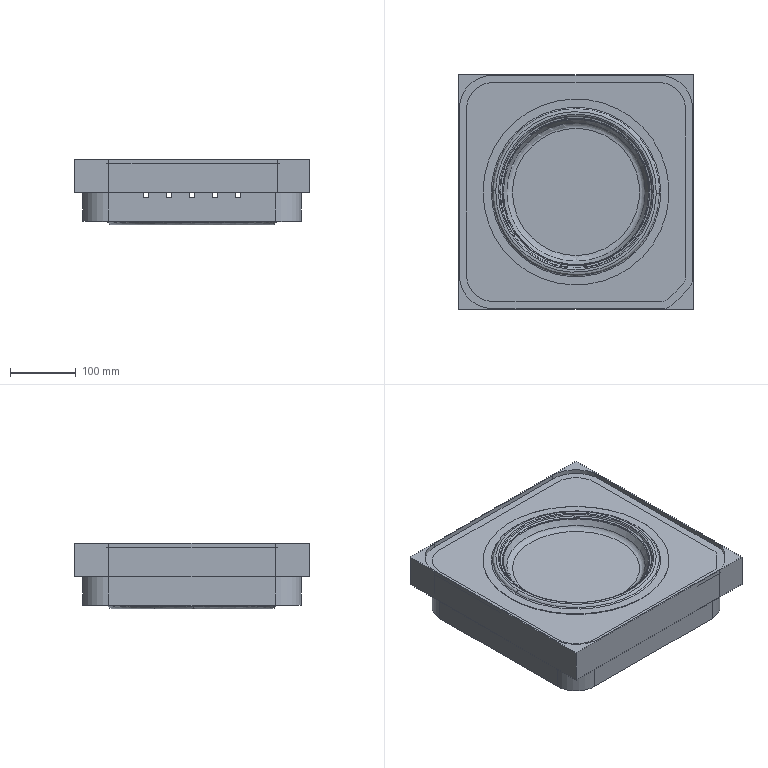NC program | NX | posted with a generic post | part box 356 x 356 x 99.5 mm
Lines 5552 to 6475 of 165566:
(06 , TOOL : R2)
N11090 M6
N11092 G53
N11094 G17 G0 G90 X-7.96 Y-140.743 S8000 M3 M8
N11096 G43 Z200.5 H0
N11098 Z47.725
N11100 G94 G1 Z44.725 F4500.
N11102 X-8.307 Y-140.727
N11104 X-8.475 Y-140.721
N11106 X-10.032 Y-140.636
N11108 G2 X-20.418 Y-139.492 R132.954
N11110 G1 X-21.112 Y-139.397
N11112 X-21.594 Y-139.336
N11114 X-26.993 Y-138.383
N11116 X-27.456 Y-138.297
N11118 X-32.877 Y-137.105
N11120 X-33.572 Y-136.93
N11122 X-33.644 Y-136.913
N11124 X-37.606 Y-135.874
N11126 X-38.416 Y-135.657
N11128 X-38.877 Y-135.528
N11130 X-42.571 Y-134.392
N11132 X-43.388 Y-134.143
N11134 X-43.954 Y-133.964
N11136 X-44.464 Y-133.797
N11138 X-49.379 Y-132.066
N11140 X-50.266 Y-131.72
N11142 X-50.877 Y-131.476
N11144 X-53.992 Y-130.232
N11146 G2 X-57.735 Y-128.604 R67.091
N11148 G1 X-60.048 Y-127.566
N11150 X-60.222 Y-127.485
N11152 X-60.567 Y-127.317
N11154 X-65.412 Y-124.904
N11156 X-65.76 Y-124.713
N11158 X-68.399 Y-123.263
N11160 X-69.566 Y-122.621
N11162 X-70.632 Y-122.027
N11164 X-71.206 Y-121.68
N11166 X-75.449 Y-119.111
N11168 X-76.798 Y-118.218
N11170 X-77.32 Y-117.873
N11172 X-77.841 Y-117.527
N11174 X-78.22 Y-117.277
N11176 X-78.889 Y-116.834
N11178 X-78.913 Y-116.818
N11180 X-79.93 Y-116.145
N11182 X-80.442 Y-115.796
N11184 X-82.356 Y-114.411
N11186 X-84.747 Y-112.68
N11188 X-85.207 Y-112.334
N11190 X-86.523 Y-111.293
N11192 X-87.216 Y-110.748
N11194 X-88.28 Y-109.911
N11196 X-89.16 Y-109.218
N11198 X-89.592 Y-108.872
N11200 X-90.603 Y-108.006
N11202 X-93.632 Y-105.41
N11204 X-94.026 Y-105.064
N11206 X-94.142 Y-104.957
N11208 X-94.772 Y-104.37
N11210 X-95.492 Y-103.701
N11212 X-95.869 Y-103.35
N11214 X-96.217 Y-103.026
N11216 X-96.259 Y-102.987
N11218 X-98.119 Y-101.256
N11220 X-102.231 Y-97.102
N11222 X-102.746 Y-96.538
N11224 X-105.074 Y-93.985
N11226 X-106.021 Y-92.948
N11228 X-106.601 Y-92.267
N11230 X-107.77 Y-90.874
N11232 X-109.802 Y-88.448
N11234 X-111.945 Y-85.679
N11236 X-113.279 Y-83.947
N11238 X-113.529 Y-83.608
N11240 X-113.778 Y-83.255
N11242 X-114.519 Y-82.209
N11244 X-115.248 Y-81.179
N11246 X-115.253 Y-81.172
N11248 X-116.227 Y-79.794
N11250 X-116.717 Y-79.101
N11252 X-119.859 Y-74.255
N11254 X-120.476 Y-73.216
N11256 X-121.829 Y-70.929
N11258 X-121.909 Y-70.793
N11260 X-121.959 Y-70.708 Z44.724
N11262 X-122.108 Y-70.453 Z44.725
N11264 X-122.174 Y-70.344
N11266 X-122.518 Y-69.76
N11268 X-122.867 Y-69.164
N11270 X-122.921 Y-69.062
N11272 X-123.906 Y-67.231
N11274 X-124.965 Y-65.254
N11276 X-125.522 Y-64.216
N11278 X-125.691 Y-63.878
N11280 X-128.048 Y-59.023
N11282 X-128.654 Y-57.639
N11284 X-130.312 Y-53.83
N11286 X-130.478 Y-53.432
N11288 X-131.665 Y-50.369
N11290 X-132.466 Y-48.291
N11292 X-132.591 Y-47.945
N11294 X-134.357 Y-42.753
N11296 X-135.18 Y-39.983
N11298 X-135.877 Y-37.62
N11300 X-135.996 Y-37.214
N11302 X-136.016 Y-37.139
N11304 X-137.392 Y-31.675
N11306 X-137.402 Y-31.632
N11308 X-138.548 Y-26.136
N11310 X-138.673 Y-25.444
N11312 X-139.133 Y-22.68
N11314 X-139.475 Y-20.597
N11316 X-139.495 Y-20.562
N11318 X-140.18 Y-15.059
N11320 X-140.26 Y-14.366
N11322 X-140.717 Y-8.827
N11324 X-140.738 Y-8.481
N11326 X-140.794 Y-7.097
N11328 X-140.865 Y-5.468
N11330 Y-5.366
N11332 X-140.88 Y-5.02
N11334 X-140.881 Y-5.012
N11336 X-140.896 Y-4.673
N11338 X-140.965 Y-2.942
N11340 X-140.982 Y-1.558
N11342 X-140.989 Y-0.865
N11344 X-140.994 Y-0.173
N11346 X-140.993 Y0.516
N11348 X-140.985 Y1.212
N11350 X-140.978 Y1.904
N11352 X-140.965 Y2.934
N11354 X-140.951 Y3.289
N11356 G3 X-140.738 Y8.477 R4785.324
N11358 G1 X-140.691 Y9.172
N11360 X-140.261 Y14.355
N11362 G2 X-139.475 Y20.597 R236.107
N11364 G1 X-138.731 Y25.098
N11366 X-138.614 Y25.788
N11368 X-138.549 Y26.131
N11370 X-137.404 Y31.632
N11372 X-137.219 Y32.366
N11374 X-136.017 Y37.136
N11376 X-135.996 Y37.214
N11378 X-135.895 Y37.56
N11380 X-135.086 Y40.303
N11382 X-134.358 Y42.748
N11384 X-132.558 Y48.043
N11386 X-132.336 Y48.637
N11388 X-130.481 Y53.425
N11390 X-130.313 Y53.828
N11392 X-128.204 Y58.675
N11394 X-128.052 Y59.014
N11396 X-127.209 Y60.753
N11398 X-125.982 Y63.28
N11400 X-125.636 Y63.994
N11402 X-125.521 Y64.213
N11404 X-124.966 Y65.254
N11406 X-122.867 Y69.165
N11408 X-122.726 Y69.407
N11410 X-120.45 Y73.261
N11412 X-119.86 Y74.253
N11414 X-116.718 Y79.1
N11416 X-116.29 Y79.706
N11418 X-115.599 Y80.686
N11420 X-115.491 Y80.833
N11422 X-114.56 Y82.152
N11424 X-113.867 Y83.13
N11426 X-113.525 Y83.613
N11428 X-113.176 Y84.083
N11430 X-112.484 Y84.981
N11432 X-112.479 Y84.986
N11434 X-110.072 Y88.1
N11436 X-109.971 Y88.23 Z44.723
N11438 X-109.801 Y88.448 Z44.725
N11440 X-107.293 Y91.443
N11442 X-107.19 Y91.564
N11444 X-106.946 Y91.855
N11446 X-106.611 Y92.253
N11448 X-106.254 Y92.678
N11450 X-106.021 Y92.947
N11452 X-105.907 Y93.072
N11454 X-105.074 Y93.987
N11456 X-104.178 Y94.97
N11458 X-102.867 Y96.408
N11460 X-102.447 Y96.87
N11462 X-102.101 Y97.237
N11464 X-98.12 Y101.255
N11466 X-94.487 Y104.637
N11468 X-94.027 Y105.064
N11470 X-93.449 Y105.566
N11472 X-92.756 Y106.162
N11474 X-89.592 Y108.872
N11476 X-88.722 Y109.565
N11478 X-86.964 Y110.948
N11480 X-86.872 Y111.02
N11482 X-85.042 Y112.458 Z44.723
N11484 X-84.796 Y112.642 Z44.725
N11486 X-84.795 Y112.643
N11488 X-82.356 Y114.411
N11490 X-81.357 Y115.132
N11492 X-80.296 Y115.898
N11494 X-75.451 Y119.11
N11496 X-75.105 Y119.319
N11498 X-72.976 Y120.609
N11500 X-72.352 Y120.988
N11502 X-70.605 Y122.043
N11504 X-66.874 Y124.104
N11506 X-66.287 Y124.425
N11508 X-66.106 Y124.526
N11510 X-66.012 Y124.577 Z44.724
N11512 X-65.76 Y124.714 Z44.725
N11514 X-65.414 Y124.903
N11516 X-60.915 Y127.144
N11518 X-60.568 Y127.316
N11520 X-60.056 Y127.562
N11522 X-56.961 Y128.951
N11524 X-56.416 Y129.194
N11526 X-55.39 Y129.653
N11528 X-54.603 Y129.989
N11530 X-50.877 Y131.476
N11532 X-49.38 Y132.063
N11534 X-49.146 Y132.147
N11536 X-46.432 Y133.105
N11538 X-44.301 Y133.851
N11540 X-43.387 Y134.143
N11542 X-39.456 Y135.348
N11544 X-38.763 Y135.56
N11546 X-38.072 Y135.75
N11548 X-37.379 Y135.933
N11550 X-35.306 Y136.475
N11552 X-33.918 Y136.842
N11554 X-32.88 Y137.105
N11556 X-27.456 Y138.297
N11558 X-26.996 Y138.383
N11560 X-24.227 Y138.871
N11562 X-22.843 Y139.114
N11564 X-21.593 Y139.336
N11566 X-21.115 Y139.396
N11568 X-16.267 Y140.05
N11570 X-15.575 Y140.128
N11572 X-10.729 Y140.579
N11574 X-10.037 Y140.635
N11576 X-8.474 Y140.721
N11578 X-7.963 Y140.743
N11580 X-7.268 Y140.78
N11582 X-6.23 Y140.833
N11584 X-4.499 Y140.919
N11586 X-3.807 Y140.936
N11588 X-2.769 Y140.946
N11590 X1.038 Y140.986
N11592 X1.384 Y140.983
N11594 X1.726 Y140.977
N11596 X6.23 Y140.845
N11598 X6.918 Y140.822
N11600 X7.609 Y140.784
N11602 X8.534 Y140.721
N11604 X8.999 Y140.684
N11606 X9.345 Y140.659
N11608 X10.383 Y140.585
N11610 X11.768 Y140.484
N11612 X12.791 Y140.411
N11614 X13.221 Y140.374
N11616 X18.681 Y139.751
N11618 X19.171 Y139.682
N11620 X24.224 Y138.896
N11622 X24.57 Y138.836
N11624 X26.302 Y138.496
N11626 X30.105 Y137.743
N11628 X30.706 Y137.605
N11630 X35.646 Y136.413
N11632 X35.99 Y136.322
N11634 X36.341 Y136.22
N11636 X36.357 Y136.219
N11638 X36.375 Y136.215
N11640 X41.224 Y134.836
N11642 X42.291 Y134.491
N11644 X46.489 Y133.105
N11646 X47.46 Y132.759
N11648 X50.185 Y131.736
N11650 X52.057 Y131.028
N11652 X52.91 Y130.681
N11654 X53.727 Y130.334
N11656 X56.152 Y129.31
N11658 X57.778 Y128.614
N11660 X57.794 Y128.604
N11662 X58.149 Y128.437
N11664 X59.532 Y127.783
N11666 X62.191 Y126.526
N11668 X62.915 Y126.181
N11670 X64.24 Y125.489
N11672 X67.536 Y123.762
N11674 X68.183 Y123.412
N11676 X72.979 Y120.642
N11678 X73.72 Y120.172
N11680 X77.893 Y117.528
N11682 X78.398 Y117.18
N11684 X79.398 Y116.487
N11686 X79.896 Y116.141
N11688 X82.717 Y114.183
N11690 X82.875 Y114.064
N11692 X83.397 Y113.67
N11694 X87.002 Y110.949
N11696 X87.44 Y110.603
N11698 X87.911 Y110.216
N11700 X89.127 Y109.217
N11702 X89.968 Y108.526
N11704 X91.653 Y107.141
N11706 X92.047 Y106.795
N11708 X94.833 Y104.308
N11710 X95.149 Y104.026
N11712 X95.175 Y104.002
N11714 X95.925 Y103.333
N11716 X96.216 Y103.063
N11718 X100.218 Y99.179
N11720 X102.847 Y96.41
N11722 X104.167 Y95.025
N11724 X107.492 Y91.225
N11726 X108.097 Y90.525
N11728 X111.44 Y86.372
N11730 X111.71 Y86.024
N11732 X113.247 Y83.948
N11734 X115.036 Y81.524
N11736 X115.252 Y81.216
N11738 X115.512 Y80.831
N11740 X115.945 Y80.194
N11742 X118.365 Y76.614
N11744 X119.406 Y74.936
N11746 X119.54 Y74.718
N11748 X121.324 Y71.832
N11750 X121.526 Y71.485
N11752 X124.256 Y66.639
N11754 X124.341 Y66.471 Z44.722
N11756 X124.43 Y66.294 Z44.725
N11758 X124.608 Y65.947
N11760 X125.49 Y64.22
N11762 X126.728 Y61.792
N11764 X127.02 Y61.192
N11766 X128.55 Y57.865
N11768 X128.972 Y56.945
N11770 X129.284 Y56.254
N11772 X130.135 Y54.198
N11774 X130.142 Y54.177
N11776 X130.286 Y53.83
N11778 X131.282 Y51.407
N11780 X131.558 Y50.715
N11782 X132.061 Y49.33
N11784 X132.439 Y48.292
N11786 X132.903 Y47.015
N11788 X133.164 Y46.302
N11790 X133.25 Y46.063
N11792 X133.443 Y45.522
N11794 X133.779 Y44.484
N11796 X134.992 Y40.675
N11798 X135.206 Y39.983
N11800 X135.672 Y38.296
N11802 X136.712 Y34.498
N11804 X136.806 Y34.098
N11806 X137.996 Y28.906
N11808 X138.096 Y28.435
N11810 X139.04 Y23.367
N11812 X139.101 Y23.021
N11814 X139.132 Y22.833
N11816 X139.605 Y19.559
N11818 X139.905 Y17.482
N11820 X139.948 Y17.136
N11822 X140.519 Y11.597
N11824 X140.821 Y6.75
N11826 X140.859 Y6.058
N11828 X140.876 Y6.031
N11830 X140.988 Y0.519
N11832 X140.987 Y-0.512
N11834 X140.918 Y-3.824
N11836 X140.873 Y-6.04
N11838 X140.865 Y-6.053
N11840 X140.859 Y-6.058
N11842 X140.68 Y-9.
N11844 X140.519 Y-11.597
N11846 X140.34 Y-13.328
N11848 X139.949 Y-17.13
N11850 X139.906 Y-17.475
N11852 X139.274 Y-21.846
N11854 X139.132 Y-22.83
N11856 X139.101 Y-23.021
N11858 X138.264 Y-27.521
N11860 X138.097 Y-28.43
N11862 X137.997 Y-28.903
N11864 X137.841 Y-29.596
N11866 X137.523 Y-30.983
N11868 X136.712 Y-34.496
N11870 X135.329 Y-39.553
N11872 X135.206 Y-39.981
N11874 X135.1 Y-40.33
N11876 X133.944 Y-43.964
N11878 X133.444 Y-45.52
N11880 X133.321 Y-45.868
N11882 X133.113 Y-46.437
N11884 X131.935 Y-49.676
N11886 X131.558 Y-50.714
N11888 X131.282 Y-51.407
N11890 X129.576 Y-55.553
N11892 X129.285 Y-56.251
N11894 X128.972 Y-56.946
N11896 X128.653 Y-57.641
N11898 X128.201 Y-58.625
N11900 X127.021 Y-61.191
N11902 X126.901 Y-61.445
N11904 X126.674 Y-61.906
N11906 X126.555 Y-62.139
N11908 X124.255 Y-66.641
N11910 X124.062 Y-66.985
N11912 X123.477 Y-68.024
N11914 X121.525 Y-71.48
N11916 X121.325 Y-71.83
N11918 X121.134 Y-72.14
N11920 X120.899 Y-72.523
N11922 X120.445 Y-73.259
N11924 X120.327 Y-73.448
N11926 X119.827 Y-74.255
N11928 X119.406 Y-74.935
N11930 X118.368 Y-76.612
N11932 X116.637 Y-79.171
N11934 X116.214 Y-79.794
N11936 X115.945 Y-80.193
N11938 X115.512 Y-80.831
N11940 X115.253 Y-81.215
N11942 X115.036 Y-81.524
N11944 X114.561 Y-82.173
N11946 X112.483 Y-84.982
N11948 X111.792 Y-85.916
N11950 X111.445 Y-86.367
N11952 X108.098 Y-90.524
N11954 X107.985 Y-90.66
N11956 X106.6 Y-92.243
N11958 X104.524 Y-94.619
N11960 X104.47 Y-94.679
N11962 X104.177 Y-95.014
N11964 X100.219 Y-99.179
N11966 X96.217 Y-103.062
N11968 X95.925 Y-103.334
N11970 X95.871 Y-103.382
N11972 X91.718 Y-107.087
N11974 X91.074 Y-107.62
N11976 X89.711 Y-108.739
N11978 X88.603 Y-109.651
N11980 X87.218 Y-110.781
N11982 X86.542 Y-111.296
N11984 X85.169 Y-112.334
N11986 X82.719 Y-114.182
N11988 X81.743 Y-114.861
N11990 X81.335 Y-115.144
N11992 X79.894 Y-116.142
N11994 X78.912 Y-116.823
N11996 X78.566 Y-117.062
N11998 X78.55 Y-117.073
N12000 X77.895 Y-117.527
N12002 X77.874 Y-117.541
N12004 X77.734 Y-117.63 Z44.722
N12006 X77.531 Y-117.759 Z44.725
N12008 X72.98 Y-120.642
N12010 X69.57 Y-122.611
N12012 X68.848 Y-123.027
N12014 X68.183 Y-123.412
N12016 X67.151 Y-123.963
N12018 X62.991 Y-126.142
N12020 X62.916 Y-126.179
N12022 G2 X57.454 Y-128.756 R593.172
N12024 G1 X56.415 Y-129.198
N12026 X53.646 Y-130.368
N12028 X52.914 Y-130.68
N12030 X52.495 Y-130.853
N12032 X52.262 Y-130.948
N12034 X52.07 Y-131.023
N12036 X50.531 Y-131.605
N12038 X47.07 Y-132.901
N12040 X46.724 Y-133.024
N12042 X46.499 Y-133.101
N12044 X44.393 Y-133.795
N12046 X42.917 Y-134.284
N12048 X41.224 Y-134.836
N12050 X36.357 Y-136.219
N12052 X36.341 Y-136.22
N12054 X35.995 Y-136.321
N12056 X35.649 Y-136.412
N12058 X35.021 Y-136.566
N12060 X30.711 Y-137.604
N12062 X30.111 Y-137.742
N12064 X24.573 Y-138.836
N12066 X23.638 Y-138.989
N12068 X19.382 Y-139.649
N12070 X19.172 Y-139.68
N12072 X18.69 Y-139.75
N12074 X14.883 Y-140.184
N12076 X14.19 Y-140.261
N12078 X13.222 Y-140.374
N12080 X12.806 Y-140.41
N12082 X7.614 Y-140.784
N12084 X6.922 Y-140.822
N12086 X6.23 Y-140.845
N12088 X1.731 Y-140.977
N12090 X1.384 Y-140.983
N12092 X1.038 Y-140.986
N12094 X-3.805 Y-140.936
N12096 X-4.497 Y-140.92
N12098 X-7.96 Y-140.743
N12100 Y-140.458
N12102 X-8.626 Y-140.427
N12104 G2 X-16.594 Y-139.719 R116.439
N12106 G1 X-21.487 Y-139.061
N12108 X-26.996 Y-138.092
N12110 X-27.342 Y-138.028
N12112 G2 X-49.482 Y-131.72 R141.758
N12114 G1 X-50.185 Y-131.445
N12116 G2 X-70.605 Y-121.71 R138.589
N12118 G1 X-71.797 Y-120.989
N12120 X-72.133 Y-120.786
N12122 X-75.227 Y-118.911
N12124 G2 X-102.101 Y-96.821 R141.205
N12126 G1 X-102.628 Y-96.245
N12128 X-105.764 Y-92.804
N12130 X-106.529 Y-91.91
N12132 X-109.419 Y-88.463
N12134 X-109.559 Y-88.291
N12136 X-109.709 Y-88.102
N12138 X-112.064 Y-85.057
N12140 X-113.176 Y-83.606
N12142 X-114.899 Y-81.178
N12144 X-115.045 Y-80.973
N12146 X-116.353 Y-79.122
N12148 X-116.478 Y-78.941
N12150 X-116.602 Y-78.755
N12152 X-119.609 Y-74.112
N12154 X-120.91 Y-71.925
N12156 X-121.578 Y-70.793
N12158 X-121.829 Y-70.366
N12160 X-122.596 Y-69.062
N12162 X-125.29 Y-64.042
N12164 X-126.701 Y-61.147
N12166 X-127.053 Y-60.423
N12168 X-127.722 Y-59.042
N12170 X-127.838 Y-58.795
N12172 G2 X-134.056 Y-42.753 R142.682
N12174 G1 X-135.29 Y-38.599
N12176 X-135.7 Y-37.214
N12178 X-136.187 Y-35.304
N12180 X-137.099 Y-31.675
N12182 G2 X-140.452 Y-8.481 R142.554
N12184 G1 X-140.455 Y-8.418
N12186 X-140.538 Y-6.427
N12188 X-140.592 Y-5.093
N12190 G2 X-140.583 Y5.302 R110.795
N12192 G1 X-140.58 Y5.366
N12194 X-140.57 Y5.675
N12196 X-140.447 Y8.553
N12198 X-140.394 Y9.298
N12200 X-139.989 Y14.204
N12202 X-139.853 Y15.384
N12204 X-139.235 Y20.35
N12206 X-139.187 Y20.597
N12208 X-139.178 Y20.65
N12210 X-138.442 Y25.095
N12212 X-138.295 Y25.937
N12214 X-137.827 Y28.213
N12216 X-137.1 Y31.67
N12218 X-135.771 Y36.944
N12220 X-135.702 Y37.207
N12222 X-134.109 Y42.587
N12224 X-133.25 Y45.124
N12226 G2 X-130. Y53.83 R125.039
N12228 G1 X-127.838 Y58.794
N12230 X-126.388 Y61.792
N12232 X-125.982 Y62.625
N12234 X-125.547 Y63.523
N12236 X-125.379 Y63.869
N12238 X-125.365 Y63.896
N12240 X-125.096 Y64.409
N12242 X-125.016 Y64.562
N12244 X-122.586 Y69.081
N12246 X-120.213 Y73.101
N12248 X-119.704 Y73.957
N12250 X-119.518 Y74.255
N12252 X-119.492 Y74.296
N12254 X-116.535 Y78.857
N12256 X-116.354 Y79.122
N12258 X-115.351 Y80.542
N12260 X-113.179 Y83.602
N12262 X-112.9 Y83.975
N12264 X-109.689 Y88.128
N12266 X-109.43 Y88.448
N12268 X-109.073 Y88.875
N12270 X-105.918 Y92.631
N12272 X-103.95 Y94.796
N12274 X-102.118 Y96.803
N12276 G2 X-91.577 Y106.795 R131.576
N12278 G1 X-90.132 Y108.035
N12280 X-89.415 Y108.649
N12282 X-88.663 Y109.247
N12284 G2 X-74.087 Y119.604 R134.667
N12286 G1 X-73.438 Y119.998
N12288 X-72.759 Y120.408
N12290 X-72.28 Y120.699
N12292 X-70.532 Y121.755
N12294 X-68.529 Y122.866
N12296 X-65.414 Y124.578
N12298 G2 X-10.441 Y140.316 R141.001
N12300 G1 X-10.064 Y140.347
N12302 X-8.339 Y140.441
N12304 G2 X7.73 Y140.49 R137.262
N12306 X19.036 Y139.413 R134.033
N12308 G1 X23.189 Y138.768
N12310 X23.535 Y138.715
N12312 X24.195 Y138.611
N12314 G2 X47.416 Y132.47 R139.657
N12316 G1 X49.186 Y131.807
N12318 X50.185 Y131.431
N12320 X52.165 Y130.681
N12322 X54.761 Y129.588
N12324 X57.584 Y128.391
N12326 G2 X77.874 Y117.196 R142.328
N12328 G1 X82.581 Y113.927
N12330 G2 X95.871 Y102.995 R142.11
N12332 G1 X100.072 Y98.919
N12334 X103.968 Y94.82
N12336 G2 X114.929 Y81.181 R142.124
N12338 G1 X115.061 Y80.987
N12340 X116.459 Y78.923
N12342 X116.752 Y78.491
N12344 X118.022 Y76.616
N12346 X118.142 Y76.431
N12348 X118.368 Y76.067
N12350 X119.326 Y74.521
N12352 X120.114 Y73.251
N12354 X120.252 Y73.024
N12356 X121.165 Y71.538
N12358 X123.298 Y67.761
N12360 X123.921 Y66.652
N12362 G2 X126.907 Y60.754 R133.035
N12364 G1 X127.051 Y60.443
N12366 X127.161 Y60.202
N12368 G2 X134.47 Y41.368 R134.33
N12370 G1 X134.691 Y40.681
N12372 X134.761 Y40.456
N12374 X134.981 Y39.727
N12376 X136.428 Y34.454
N12378 X137.389 Y30.29
N12380 X137.712 Y28.868
N12382 X137.777 Y28.565
N12384 X138.817 Y23.005
N12386 X139.616 Y17.482
N12388 X139.697 Y16.79
N12390 X140.232 Y11.602
N12392 X140.535 Y6.77
N12394 X140.571 Y6.114
N12396 X140.575 Y6.058
N12398 X140.595 Y5.789
N12400 G2 X140.571 Y-6.114 R144.764
N12402 G1 X140.317 Y-10.25
N12404 X140.237 Y-11.533
N12406 X140.232 Y-11.597
N12408 X139.66 Y-17.136
N12410 X139.561 Y-17.879
N12412 X138.818 Y-23.004
N12414 X137.78 Y-28.549
N12416 X137.548 Y-29.598
N12418 G2 X123.96 Y-66.585 R140.355
N12420 G1 X121.59 Y-70.793
N12422 X121.137 Y-71.585
N12424 X120.121 Y-73.239
N12426 X118.145 Y-76.431
N12428 X116.34 Y-79.101
N12430 X115.945 Y-79.682
N12432 X115.637 Y-80.14
N12434 X114.915 Y-81.2
N12436 X114.215 Y-82.162
N12438 X111.556 Y-85.755
N12440 X111.241 Y-86.164
N12442 X107.999 Y-90.192
N12444 X107.723 Y-90.525
N12446 X107.702 Y-90.55
N12448 X103.971 Y-94.817
N12450 X100.024 Y-98.968
N12452 X99.808 Y-99.179
N12454 X96.241 Y-102.641
N12456 X95.879 Y-102.987
N12458 X95.771 Y-103.088
N12460 X91.496 Y-106.9
N12462 X90.786 Y-107.488
N12464 X89.411 Y-108.617
N12466 X88.257 Y-109.565
N12468 X87.218 Y-110.413
N12470 X86.981 Y-110.603
N12472 G2 X72.79 Y-120.422 R141.261
N12474 G1 X70.466 Y-121.764
N12476 X68.142 Y-123.106
N12478 X67.837 Y-123.274
N12480 X67.144 Y-123.645
N12482 X62.964 Y-125.835
N12484 X62.027 Y-126.289
N12486 X59.325 Y-127.566
N12488 X57.827 Y-128.272
N12490 X57.587 Y-128.39
N12492 G2 X42.64 Y-134.074 R138.767
N12494 G1 X41.193 Y-134.546
N12496 X41.102 Y-134.574
N12498 X36.346 Y-135.927
N12500 X36.27 Y-135.945
N12502 X35.995 Y-136.023
N12504 X35.324 Y-136.199
N12506 X30.313 Y-137.403
N12508 X29.419 Y-137.59
N12510 X28.145 Y-137.84
N12512 X27.713 Y-137.927
N12514 X27.343 Y-138.002
N12516 X26.85 Y-138.097
N12518 X24.573 Y-138.544
N12520 G2 X17.651 Y-139.583 R164.141
N12522 G1 X16.633 Y-139.697
N12524 X16.268 Y-139.742
N12526 X13.165 Y-140.093
N12528 X10.729 Y-140.274
N12530 X7.483 Y-140.506
N12532 G2 X-7.96 Y-140.458 R133.056
N12534 G1 Y-140.173
N12536 X-10.035 Y-140.063
N12538 G2 X-27.162 Y-137.771 R140.887
N12540 G1 X-28.727 Y-137.435
N12542 G2 X-65.06 Y-124.442 R139.684
N12544 G1 X-66.798 Y-123.494
N12546 X-70.196 Y-121.618
N12548 X-70.605 Y-121.377
N12550 G2 X-97.653 Y-100.91 R141.185
N12552 G1 X-98.899 Y-99.657
N12554 X-101.755 Y-96.772
N12556 X-104.224 Y-94.071
N12558 X-105.562 Y-92.605
N12560 X-105.862 Y-92.256
N12562 X-106.201 Y-91.857
N12564 X-109.347 Y-88.102
N12566 G2 X-113.12 Y-83.199 R254.493
N12568 X-122.358 Y-68.899 R139.269
N12570 G1 X-125.011 Y-63.961
N12572 G2 X-138.984 Y20.055 R140.594
N12574 G1 X-138.883 Y20.684
N12576 X-138.096 Y25.433
N12578 X-138.033 Y25.79
N12580 X-138.018 Y25.868
N12582 X-137.57 Y28.047
N12584 X-136.834 Y31.553
N12586 G2 X-132.945 Y45.135 R133.136
N12588 X-124.8 Y64.359 R134.468
N12590 G1 X-122.388 Y68.849
N12592 X-121.86 Y69.754
N12594 X-119.607 Y73.562
N12596 X-119.399 Y73.909
N12598 X-117.609 Y76.678
N12600 X-116.711 Y78.063
N12602 X-116.291 Y78.709
N12604 X-114.907 Y80.673
N12606 X-113.077 Y83.255
N12608 G2 X-79.983 Y115.417 R140.645
N12610 G1 X-78.566 Y116.365
N12612 G2 X-65.688 Y124.104 R130.484
N12614 G1 X-65.043 Y124.45
N12616 X-60.178 Y126.874
N12618 G2 X-38.581 Y135.018 R144.891
N12620 X-21.305 Y138.797 R142.186
N12622 G1 X-16.109 Y139.494
N12624 X-15.333 Y139.577
N12626 X-10.729 Y140.006
N12628 X-10.037 Y140.063
N12630 X-7.077 Y140.219
N12632 X-4.527 Y140.347
N12634 X-4.171 Y140.357
N12636 X-3.816 Y140.365
N12638 G2 X24.34 Y138.297 R139.868
N12640 G1 X25.956 Y137.983
N12642 G2 X53.235 Y129.924 R136.993
N12644 G1 X57.453 Y128.135
N12646 X62.538 Y125.728
N12648 G2 X99.755 Y98.833 R140.347
N12650 G1 X103.708 Y94.679
N12652 X107.293 Y90.584
N12654 X107.639 Y90.183
N12656 X111.037 Y85.962
N12658 X111.446 Y85.424
N12660 X114.561 Y81.208
N12662 X115.253 Y80.198
N12664 X117.866 Y76.332
N12666 X120.791 Y71.611
N12668 G2 X128.787 Y55.964 R143.035
N12670 G1 X129.789 Y53.539
N12672 X130.665 Y51.407
N12674 G2 X133.25 Y44.266 R114.365
N12676 G1 X133.401 Y43.791
N12678 X134.502 Y40.33
N12680 X134.635 Y39.9
N12682 G2 X138.523 Y23.021 R143.444
N12684 G1 X138.73 Y21.636
N12686 G2 X140.254 Y-6.669 R140.079
N12688 X136.174 Y-34.289 R141.381
N12690 X114.58 Y-81.178 R140.745
N12692 G1 X112.657 Y-83.787
N12694 X111.446 Y-85.425
N12696 X111.254 Y-85.679
N12698 X110.754 Y-86.316
N12700 X107.649 Y-90.168
N12702 G2 X86.872 Y-110.324 R140.373
N12704 G1 X85.151 Y-111.632
N12706 X82.35 Y-113.742
N12708 G2 X24.23 Y-138.316 R140.499
N12710 X-4.474 Y-140.349 R141.055
N12712 G1 X-7.96 Y-140.173
N12714 X-7.947 Y-139.889
N12716 X-10.037 Y-139.776
N12718 X-10.125 Y-139.77
N12720 G2 X-109.256 Y-87.756 R140.11
N12722 G1 X-111.634 Y-84.681
N12724 X-112.726 Y-83.255
N12726 G2 X-124.807 Y-63.732 R140.143
N12728 G1 X-126.168 Y-60.939
N12730 X-127.296 Y-58.606
N12732 X-128.665 Y-55.475
N12734 X-129.606 Y-53.3
N12736 G2 X-135.641 Y-35.137 R135.606
N12738 G1 X-136.549 Y-31.513
N12740 X-137.243 Y-28.213
N12742 X-137.687 Y-26.074
N12744 X-137.864 Y-25.098
N12746 X-138.685 Y-20.148
N12748 G2 X-139.428 Y14.072 R141.
N12750 G1 X-139.319 Y15.059
N12752 G2 X-137.293 Y27.978 R128.815
N12754 G1 X-136.558 Y31.483
N12756 G2 X-122.085 Y68.806 R141.115
N12758 G1 X-120.507 Y71.485
N12760 X-119.274 Y73.562
N12762 X-119.063 Y73.905
N12764 G2 X-89.083 Y108.18 R140.845
N12766 G1 X-87.911 Y109.114
N12768 G2 X-65.045 Y124.127 R138.805
N12770 X-59.552 Y126.851 R341.742
N12772 X-21.459 Y138.487 R141.019
N12774 G1 X-16.042 Y139.215
N12776 G2 X41.038 Y133.995 R140.066
N12778 G1 X42.085 Y133.658
N12780 X46.507 Y132.195
N12782 G2 X67.327 Y122.902 R142.14
N12784 G1 X67.665 Y122.719
N12786 X67.837 Y122.623
N12788 X72.467 Y119.95
N12790 X77.389 Y116.834
N12792 X79.95 Y115.062
N12794 X82.172 Y113.518
N12796 X82.372 Y113.373
N12798 X83.411 Y112.588
N12800 X86.514 Y110.245
N12802 G2 X96.565 Y101.532 R132.443
N12804 G1 X99.678 Y98.506
N12806 G2 X117.585 Y76.241 R140.394
N12808 G1 X119.828 Y72.625
N12810 X120.629 Y71.324
N12812 X120.757 Y71.106
N12814 X120.875 Y70.899
N12816 G2 X129.48 Y53.541 R134.037
N12818 G1 X130.591 Y50.831
N12820 X130.828 Y50.22
N12822 X132.632 Y45.249
N12824 G2 X134.462 Y39.464 R433.306
N12826 G1 X135.876 Y34.302
N12828 G2 X140.023 Y-5.712 R140.305
N12830 G1 X139.839 Y-8.754
N12832 X139.657 Y-11.597
N12834 X139.079 Y-17.19
N12836 X138.692 Y-19.905
N12838 X138.263 Y-22.853
N12840 X137.231 Y-28.386
N12842 X136.963 Y-29.598
N12844 X135.898 Y-34.219
N12846 X134.414 Y-39.637
N12848 X134.321 Y-39.951
N12850 G2 X95.179 Y-102.852 R140.017
N12852 X-4.497 Y-140.064 R140.162
N12854 G1 X-7.947 Y-139.889
N12856 X-7.933 Y-139.604
N12858 X-9.858 Y-139.502
N12860 G2 X-74.744 Y-118.204 R139.987
N12862 G1 X-76.143 Y-117.284
N12864 G2 X-93.448 Y-104.044 R136.464
N12866 G1 X-97.223 Y-100.532
N12868 X-97.4 Y-100.362
N12870 X-101.359 Y-96.36
N12872 X-105.159 Y-92.199
N12874 X-106.271 Y-90.888
N12876 X-108.893 Y-87.756
N12878 X-110.614 Y-85.539
N12880 X-112.419 Y-83.191
N12882 X-112.711 Y-82.79
N12884 X-115.806 Y-78.409
N12886 X-118.855 Y-73.703
N12888 X-119.633 Y-72.404
N12890 X-121.815 Y-68.702
N12892 X-122.521 Y-67.399
N12894 X-124.477 Y-63.749
N12896 X-124.764 Y-63.177
N12898 X-127.021 Y-58.524
N12900 X-127.562 Y-57.292
N12902 G2 X-133.154 Y-42.753 R131.272
N12904 X-139.854 Y-0.204 R140.535
N12906 X-131.866 Y46.535 R139.426
N12908 G1 X-131.504 Y47.599
N12910 G2 X-93.24 Y104.235 R140.159
N12912 G1 X-91.881 Y105.411
N12914 G2 X-59.492 Y126.565 R139.113
N12916 X13.059 Y139.243 R139.854
N12918 X25.789 Y137.436 R133.005
N12920 X42.12 Y133.346 R131.558
N12922 X51.916 Y129.858 R144.789
N12924 G1 X53.907 Y129.021
N12926 X57.176 Y127.635
N12928 X62.299 Y125.211
N12930 G2 X86.304 Y110.046 R140.688